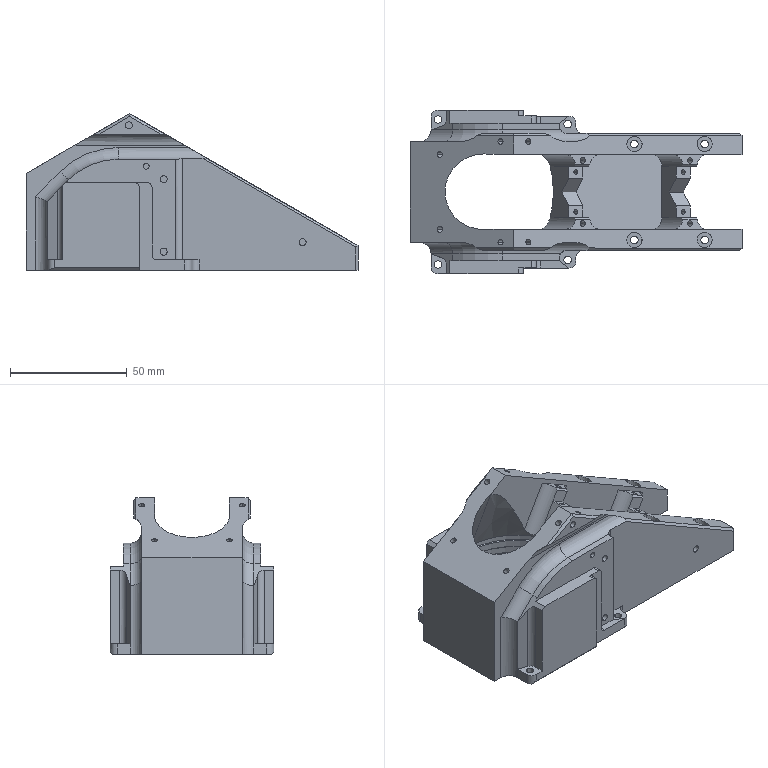NC program | NX | posted with a generic post | part box 142 x 70 x 67 mm
Lines 1 to 899 of 58889:
N10 G17 G21 G94 G90
(FACE_MILLING , TOOL : D80)
N12 T01 M6
N14 G54
N16 G17 G0 G90 X123. Y0. S2500 M3
N18 G43 Z33. H1
N20 G94 G1 Z0.3 F5000.
N22 X111. F1000.
N24 X-111.
N26 X-123.
N28 G0 Z33.
N30 M5
(DRILLING_COPY_2_COPY , TOOL : U钻-D21)
N32 T14 M6
N34 G54
N36 G17 G0 G90 X-36. Y0. S2000 M3
N38 G43 Z30. H14
N40 G94 G83 G99 Z-41. F100. Q2. R1.5
N42 G0 Z20.
N44 G80
N46 G0 X-36. Y0. Z30.
N48 M5
(PLANAR_MILL_COPY , TOOL : D16R0波刀)
N50 T02 M6
N52 G54
N54 G17 G0 G90 X87.25 Y8. S5500 M3
N56 G43 Z30.35 H2
N58 G94 G1 Z-2.65 F5000.
N60 G3 X79.25 Y0. R8. F2500.
N62 G1 Y-24.
N64 G2 X76.834 Y-29.834 R8.25
N66 G1 X75.834 Y-30.834
N68 G2 X70. Y-33.25 R8.25
N70 G1 X7.607
N72 G2 X-2.306 Y-40.729 R11.25
N74 G1 X-21.973 Y-43.25
N76 X-59.
N78 G2 X-70.25 Y-32. R11.25
N80 G1 Y-29.75
N82 X-71.
N84 G2 X-79.25 Y-21.5 R8.25
N86 G1 Y21.5
N88 G2 X-71. Y29.75 R8.25
N90 G1 X-70.25
N92 Y32.
N94 G2 X-59. Y43.25 R11.25
N96 G1 X-21.973
N98 X-2.306 Y40.729
N100 G2 X7.607 Y33.25 R11.25
N102 G1 X70.
N104 G2 X75.834 Y30.834 R8.25
N106 G1 X76.834 Y29.834
N108 G2 X79.25 Y24. R8.25
N110 G1 Y0.
N112 G3 X87.25 Y-8. R8.
N114 G0 Y8. Z-5.65
N116 G3 X79.25 Y0. R8.
N118 G1 Y-24.
N120 G2 X76.834 Y-29.834 R8.25
N122 G1 X75.834 Y-30.834
N124 G2 X70. Y-33.25 R8.25
N126 G1 X7.607
N128 G2 X-2.306 Y-40.729 R11.25
N130 G1 X-21.973 Y-43.25
N132 X-59.
N134 G2 X-70.25 Y-32. R11.25
N136 G1 Y-29.75
N138 X-71.
N140 G2 X-79.25 Y-21.5 R8.25
N142 G1 Y21.5
N144 G2 X-71. Y29.75 R8.25
N146 G1 X-70.25
N148 Y32.
N150 G2 X-59. Y43.25 R11.25
N152 G1 X-21.973
N154 X-2.306 Y40.729
N156 G2 X7.607 Y33.25 R11.25
N158 G1 X70.
N160 G2 X75.834 Y30.834 R8.25
N162 G1 X76.834 Y29.834
N164 G2 X79.25 Y24. R8.25
N166 G1 Y0.
N168 G3 X87.25 Y-8. R8.
N170 G0 Y8. Z-8.65
N172 G3 X79.25 Y0. R8.
N174 G1 Y-24.
N176 G2 X76.834 Y-29.834 R8.25
N178 G1 X75.834 Y-30.834
N180 G2 X70. Y-33.25 R8.25
N182 G1 X7.607
N184 G2 X-2.306 Y-40.729 R11.25
N186 G1 X-21.973 Y-43.25
N188 X-59.
N190 G2 X-70.25 Y-32. R11.25
N192 G1 Y-29.75
N194 X-71.
N196 G2 X-79.25 Y-21.5 R8.25
N198 G1 Y21.5
N200 G2 X-71. Y29.75 R8.25
N202 G1 X-70.25
N204 Y32.
N206 G2 X-59. Y43.25 R11.25
N208 G1 X-21.973
N210 X-2.306 Y40.729
N212 G2 X7.607 Y33.25 R11.25
N214 G1 X70.
N216 G2 X75.834 Y30.834 R8.25
N218 G1 X76.834 Y29.834
N220 G2 X79.25 Y24. R8.25
N222 G1 Y0.
N224 G3 X87.25 Y-8. R8.
N226 G0 Y8. Z-11.65
N228 G3 X79.25 Y0. R8.
N230 G1 Y-24.
N232 G2 X76.834 Y-29.834 R8.25
N234 G1 X75.834 Y-30.834
N236 G2 X70. Y-33.25 R8.25
N238 G1 X7.607
N240 G2 X-2.306 Y-40.729 R11.25
N242 G1 X-21.973 Y-43.25
N244 X-59.
N246 G2 X-70.25 Y-32. R11.25
N248 G1 Y-29.75
N250 X-71.
N252 G2 X-79.25 Y-21.5 R8.25
N254 G1 Y21.5
N256 G2 X-71. Y29.75 R8.25
N258 G1 X-70.25
N260 Y32.
N262 G2 X-59. Y43.25 R11.25
N264 G1 X-21.973
N266 X-2.306 Y40.729
N268 G2 X7.607 Y33.25 R11.25
N270 G1 X70.
N272 G2 X75.834 Y30.834 R8.25
N274 G1 X76.834 Y29.834
N276 G2 X79.25 Y24. R8.25
N278 G1 Y0.
N280 G3 X87.25 Y-8. R8.
N282 G0 Y8. Z-14.65
N284 G3 X79.25 Y0. R8.
N286 G1 Y-24.
N288 G2 X76.834 Y-29.834 R8.25
N290 G1 X75.834 Y-30.834
N292 G2 X70. Y-33.25 R8.25
N294 G1 X7.607
N296 G2 X-2.306 Y-40.729 R11.25
N298 G1 X-21.973 Y-43.25
N300 X-59.
N302 G2 X-70.25 Y-32. R11.25
N304 G1 Y-29.75
N306 X-71.
N308 G2 X-79.25 Y-21.5 R8.25
N310 G1 Y21.5
N312 G2 X-71. Y29.75 R8.25
N314 G1 X-70.25
N316 Y32.
N318 G2 X-59. Y43.25 R11.25
N320 G1 X-21.973
N322 X-2.306 Y40.729
N324 G2 X7.607 Y33.25 R11.25
N326 G1 X70.
N328 G2 X75.834 Y30.834 R8.25
N330 G1 X76.834 Y29.834
N332 G2 X79.25 Y24. R8.25
N334 G1 Y0.
N336 G3 X87.25 Y-8. R8.
N338 G0 Y8. Z-17.65
N340 G3 X79.25 Y0. R8.
N342 G1 Y-24.
N344 G2 X76.834 Y-29.834 R8.25
N346 G1 X75.834 Y-30.834
N348 G2 X70. Y-33.25 R8.25
N350 G1 X7.607
N352 G2 X-2.306 Y-40.729 R11.25
N354 G1 X-21.973 Y-43.25
N356 X-59.
N358 G2 X-70.25 Y-32. R11.25
N360 G1 Y-29.75
N362 X-71.
N364 G2 X-79.25 Y-21.5 R8.25
N366 G1 Y21.5
N368 G2 X-71. Y29.75 R8.25
N370 G1 X-70.25
N372 Y32.
N374 G2 X-59. Y43.25 R11.25
N376 G1 X-21.973
N378 X-2.306 Y40.729
N380 G2 X7.607 Y33.25 R11.25
N382 G1 X70.
N384 G2 X75.834 Y30.834 R8.25
N386 G1 X76.834 Y29.834
N388 G2 X79.25 Y24. R8.25
N390 G1 Y0.
N392 G3 X87.25 Y-8. R8.
N394 G0 Y8. Z-20.65
N396 G3 X79.25 Y0. R8.
N398 G1 Y-24.
N400 G2 X76.834 Y-29.834 R8.25
N402 G1 X75.834 Y-30.834
N404 G2 X70. Y-33.25 R8.25
N406 G1 X7.607
N408 G2 X-2.306 Y-40.729 R11.25
N410 G1 X-21.973 Y-43.25
N412 X-59.
N414 G2 X-70.25 Y-32. R11.25
N416 G1 Y-29.75
N418 X-71.
N420 G2 X-79.25 Y-21.5 R8.25
N422 G1 Y21.5
N424 G2 X-71. Y29.75 R8.25
N426 G1 X-70.25
N428 Y32.
N430 G2 X-59. Y43.25 R11.25
N432 G1 X-21.973
N434 X-2.306 Y40.729
N436 G2 X7.607 Y33.25 R11.25
N438 G1 X70.
N440 G2 X75.834 Y30.834 R8.25
N442 G1 X76.834 Y29.834
N444 G2 X79.25 Y24. R8.25
N446 G1 Y0.
N448 G3 X87.25 Y-8. R8.
N450 G0 Y8. Z-23.65
N452 G3 X79.25 Y0. R8.
N454 G1 Y-24.
N456 G2 X76.834 Y-29.834 R8.25
N458 G1 X75.834 Y-30.834
N460 G2 X70. Y-33.25 R8.25
N462 G1 X7.607
N464 G2 X-2.306 Y-40.729 R11.25
N466 G1 X-21.973 Y-43.25
N468 X-59.
N470 G2 X-70.25 Y-32. R11.25
N472 G1 Y-29.75
N474 X-71.
N476 G2 X-79.25 Y-21.5 R8.25
N478 G1 Y21.5
N480 G2 X-71. Y29.75 R8.25
N482 G1 X-70.25
N484 Y32.
N486 G2 X-59. Y43.25 R11.25
N488 G1 X-21.973
N490 X-2.306 Y40.729
N492 G2 X7.607 Y33.25 R11.25
N494 G1 X70.
N496 G2 X75.834 Y30.834 R8.25
N498 G1 X76.834 Y29.834
N500 G2 X79.25 Y24. R8.25
N502 G1 Y0.
N504 G3 X87.25 Y-8. R8.
N506 G0 Y8. Z-26.65
N508 G3 X79.25 Y0. R8.
N510 G1 Y-24.
N512 G2 X76.834 Y-29.834 R8.25
N514 G1 X75.834 Y-30.834
N516 G2 X70. Y-33.25 R8.25
N518 G1 X7.607
N520 G2 X-2.306 Y-40.729 R11.25
N522 G1 X-21.973 Y-43.25
N524 X-59.
N526 G2 X-70.25 Y-32. R11.25
N528 G1 Y-29.75
N530 X-71.
N532 G2 X-79.25 Y-21.5 R8.25
N534 G1 Y21.5
N536 G2 X-71. Y29.75 R8.25
N538 G1 X-70.25
N540 Y32.
N542 G2 X-59. Y43.25 R11.25
N544 G1 X-21.973
N546 X-2.306 Y40.729
N548 G2 X7.607 Y33.25 R11.25
N550 G1 X70.
N552 G2 X75.834 Y30.834 R8.25
N554 G1 X76.834 Y29.834
N556 G2 X79.25 Y24. R8.25
N558 G1 Y0.
N560 G3 X87.25 Y-8. R8.
N562 G0 Y8. Z-29.65
N564 G3 X79.25 Y0. R8.
N566 G1 Y-24.
N568 G2 X76.834 Y-29.834 R8.25
N570 G1 X75.834 Y-30.834
N572 G2 X70. Y-33.25 R8.25
N574 G1 X7.607
N576 G2 X-2.306 Y-40.729 R11.25
N578 G1 X-21.973 Y-43.25
N580 X-59.
N582 G2 X-70.25 Y-32. R11.25
N584 G1 Y-29.75
N586 X-71.
N588 G2 X-79.25 Y-21.5 R8.25
N590 G1 Y21.5
N592 G2 X-71. Y29.75 R8.25
N594 G1 X-70.25
N596 Y32.
N598 G2 X-59. Y43.25 R11.25
N600 G1 X-21.973
N602 X-2.306 Y40.729
N604 G2 X7.607 Y33.25 R11.25
N606 G1 X70.
N608 G2 X75.834 Y30.834 R8.25
N610 G1 X76.834 Y29.834
N612 G2 X79.25 Y24. R8.25
N614 G1 Y0.
N616 G3 X87.25 Y-8. R8.
N618 G0 Y8. Z-32.65
N620 G3 X79.25 Y0. R8.
N622 G1 Y-24.
N624 G2 X76.834 Y-29.834 R8.25
N626 G1 X75.834 Y-30.834
N628 G2 X70. Y-33.25 R8.25
N630 G1 X7.607
N632 G2 X-2.306 Y-40.729 R11.25
N634 G1 X-21.973 Y-43.25
N636 X-59.
N638 G2 X-70.25 Y-32. R11.25
N640 G1 Y-29.75
N642 X-71.
N644 G2 X-79.25 Y-21.5 R8.25
N646 G1 Y21.5
N648 G2 X-71. Y29.75 R8.25
N650 G1 X-70.25
N652 Y32.
N654 G2 X-59. Y43.25 R11.25
N656 G1 X-21.973
N658 X-2.306 Y40.729
N660 G2 X7.607 Y33.25 R11.25
N662 G1 X70.
N664 G2 X75.834 Y30.834 R8.25
N666 G1 X76.834 Y29.834
N668 G2 X79.25 Y24. R8.25
N670 G1 Y0.
N672 G3 X87.25 Y-8. R8.
N674 G0 Y8. Z-35.65
N676 G3 X79.25 Y0. R8.
N678 G1 Y-24.
N680 G2 X76.834 Y-29.834 R8.25
N682 G1 X75.834 Y-30.834
N684 G2 X70. Y-33.25 R8.25
N686 G1 X7.607
N688 G2 X-2.306 Y-40.729 R11.25
N690 G1 X-21.973 Y-43.25
N692 X-59.
N694 G2 X-70.25 Y-32. R11.25
N696 G1 Y-29.75
N698 X-71.
N700 G2 X-79.25 Y-21.5 R8.25
N702 G1 Y21.5
N704 G2 X-71. Y29.75 R8.25
N706 G1 X-70.25
N708 Y32.
N710 G2 X-59. Y43.25 R11.25
N712 G1 X-21.973
N714 X-2.306 Y40.729
N716 G2 X7.607 Y33.25 R11.25
N718 G1 X70.
N720 G2 X75.834 Y30.834 R8.25
N722 G1 X76.834 Y29.834
N724 G2 X79.25 Y24. R8.25
N726 G1 Y0.
N728 G3 X87.25 Y-8. R8.
N730 G0 Y8. Z-38.65
N732 G3 X79.25 Y0. R8.
N734 G1 Y-24.
N736 G2 X76.834 Y-29.834 R8.25
N738 G1 X75.834 Y-30.834
N740 G2 X70. Y-33.25 R8.25
N742 G1 X7.607
N744 G2 X-2.306 Y-40.729 R11.25
N746 G1 X-21.973 Y-43.25
N748 X-59.
N750 G2 X-70.25 Y-32. R11.25
N752 G1 Y-29.75
N754 X-71.
N756 G2 X-79.25 Y-21.5 R8.25
N758 G1 Y21.5
N760 G2 X-71. Y29.75 R8.25
N762 G1 X-70.25
N764 Y32.
N766 G2 X-59. Y43.25 R11.25
N768 G1 X-21.973
N770 X-2.306 Y40.729
N772 G2 X7.607 Y33.25 R11.25
N774 G1 X70.
N776 G2 X75.834 Y30.834 R8.25
N778 G1 X76.834 Y29.834
N780 G2 X79.25 Y24. R8.25
N782 G1 Y0.
N784 G3 X87.25 Y-8. R8.
N786 G0 Y8. Z-41.65
N788 G3 X79.25 Y0. R8.
N790 G1 Y-24.
N792 G2 X76.834 Y-29.834 R8.25
N794 G1 X75.834 Y-30.834
N796 G2 X70. Y-33.25 R8.25
N798 G1 X7.607
N800 G2 X-2.306 Y-40.729 R11.25
N802 G1 X-21.973 Y-43.25
N804 X-59.
N806 G2 X-70.25 Y-32. R11.25
N808 G1 Y-29.75
N810 X-71.
N812 G2 X-79.25 Y-21.5 R8.25
N814 G1 Y21.5
N816 G2 X-71. Y29.75 R8.25
N818 G1 X-70.25
N820 Y32.
N822 G2 X-59. Y43.25 R11.25
N824 G1 X-21.973
N826 X-2.306 Y40.729
N828 G2 X7.607 Y33.25 R11.25
N830 G1 X70.
N832 G2 X75.834 Y30.834 R8.25
N834 G1 X76.834 Y29.834
N836 G2 X79.25 Y24. R8.25
N838 G1 Y0.
N840 G3 X87.25 Y-8. R8.
N842 G0 Y8. Z-44.65
N844 G3 X79.25 Y0. R8.
N846 G1 Y-24.
N848 G2 X76.834 Y-29.834 R8.25
N850 G1 X75.834 Y-30.834
N852 G2 X70. Y-33.25 R8.25
N854 G1 X7.607
N856 G2 X-2.306 Y-40.729 R11.25
N858 G1 X-21.973 Y-43.25
N860 X-59.
N862 G2 X-70.25 Y-32. R11.25
N864 G1 Y-29.75
N866 X-71.
N868 G2 X-79.25 Y-21.5 R8.25
N870 G1 Y21.5
N872 G2 X-71. Y29.75 R8.25
N874 G1 X-70.25
N876 Y32.
N878 G2 X-59. Y43.25 R11.25
N880 G1 X-21.973
N882 X-2.306 Y40.729
N884 G2 X7.607 Y33.25 R11.25
N886 G1 X70.
N888 G2 X75.834 Y30.834 R8.25
N890 G1 X76.834 Y29.834
N892 G2 X79.25 Y24. R8.25
N894 G1 Y0.
N896 G3 X87.25 Y-8. R8.
N898 G0 Y8. Z-47.65
N900 G3 X79.25 Y0. R8.
N902 G1 Y-24.
N904 G2 X76.834 Y-29.834 R8.25
N906 G1 X75.834 Y-30.834
N908 G2 X70. Y-33.25 R8.25
N910 G1 X7.607
N912 G2 X-2.306 Y-40.729 R11.25
N914 G1 X-21.973 Y-43.25
N916 X-59.
N918 G2 X-70.25 Y-32. R11.25
N920 G1 Y-29.75
N922 X-71.
N924 G2 X-79.25 Y-21.5 R8.25
N926 G1 Y21.5
N928 G2 X-71. Y29.75 R8.25
N930 G1 X-70.25
N932 Y32.
N934 G2 X-59. Y43.25 R11.25
N936 G1 X-21.973
N938 X-2.306 Y40.729
N940 G2 X7.607 Y33.25 R11.25
N942 G1 X70.
N944 G2 X75.834 Y30.834 R8.25
N946 G1 X76.834 Y29.834
N948 G2 X79.25 Y24. R8.25
N950 G1 Y0.
N952 G3 X87.25 Y-8. R8.
N954 G0 Y8. Z-50.65
N956 G3 X79.25 Y0. R8.
N958 G1 Y-24.
N960 G2 X76.834 Y-29.834 R8.25
N962 G1 X75.834 Y-30.834
N964 G2 X70. Y-33.25 R8.25
N966 G1 X7.607
N968 G2 X-2.306 Y-40.729 R11.25
N970 G1 X-21.973 Y-43.25
N972 X-59.
N974 G2 X-70.25 Y-32. R11.25
N976 G1 Y-29.75
N978 X-71.
N980 G2 X-79.25 Y-21.5 R8.25
N982 G1 Y21.5
N984 G2 X-71. Y29.75 R8.25
N986 G1 X-70.25
N988 Y32.
N990 G2 X-59. Y43.25 R11.25
N992 G1 X-21.973
N994 X-2.306 Y40.729
N996 G2 X7.607 Y33.25 R11.25
N998 G1 X70.
N1000 G2 X75.834 Y30.834 R8.25
N1002 G1 X76.834 Y29.834
N1004 G2 X79.25 Y24. R8.25
N1006 G1 Y0.
N1008 G3 X87.25 Y-8. R8.
N1010 G0 Y8. Z-53.65
N1012 G3 X79.25 Y0. R8.
N1014 G1 Y-24.
N1016 G2 X76.834 Y-29.834 R8.25
N1018 G1 X75.834 Y-30.834
N1020 G2 X70. Y-33.25 R8.25
N1022 G1 X7.607
N1024 G2 X-2.306 Y-40.729 R11.25
N1026 G1 X-21.973 Y-43.25
N1028 X-59.
N1030 G2 X-70.25 Y-32. R11.25
N1032 G1 Y-29.75
N1034 X-71.
N1036 G2 X-79.25 Y-21.5 R8.25
N1038 G1 Y21.5
N1040 G2 X-71. Y29.75 R8.25
N1042 G1 X-70.25
N1044 Y32.
N1046 G2 X-59. Y43.25 R11.25
N1048 G1 X-21.973
N1050 X-2.306 Y40.729
N1052 G2 X7.607 Y33.25 R11.25
N1054 G1 X70.
N1056 G2 X75.834 Y30.834 R8.25
N1058 G1 X76.834 Y29.834
N1060 G2 X79.25 Y24. R8.25
N1062 G1 Y0.
N1064 G3 X87.25 Y-8. R8.
N1066 G0 Y8. Z-56.65
N1068 G3 X79.25 Y0. R8.
N1070 G1 Y-24.
N1072 G2 X76.834 Y-29.834 R8.25
N1074 G1 X75.834 Y-30.834
N1076 G2 X70. Y-33.25 R8.25
N1078 G1 X7.607
N1080 G2 X-2.306 Y-40.729 R11.25
N1082 G1 X-21.973 Y-43.25
N1084 X-59.
N1086 G2 X-70.25 Y-32. R11.25
N1088 G1 Y-29.75
N1090 X-71.
N1092 G2 X-79.25 Y-21.5 R8.25
N1094 G1 Y21.5
N1096 G2 X-71. Y29.75 R8.25
N1098 G1 X-70.25
N1100 Y32.
N1102 G2 X-59. Y43.25 R11.25
N1104 G1 X-21.973
N1106 X-2.306 Y40.729
N1108 G2 X7.607 Y33.25 R11.25
N1110 G1 X70.
N1112 G2 X75.834 Y30.834 R8.25
N1114 G1 X76.834 Y29.834
N1116 G2 X79.25 Y24. R8.25
N1118 G1 Y0.
N1120 G3 X87.25 Y-8. R8.
N1122 G0 Y8. Z-59.65
N1124 G3 X79.25 Y0. R8.
N1126 G1 Y-24.
N1128 G2 X76.834 Y-29.834 R8.25
N1130 G1 X75.834 Y-30.834
N1132 G2 X70. Y-33.25 R8.25
N1134 G1 X7.607
N1136 G2 X-2.306 Y-40.729 R11.25
N1138 G1 X-21.973 Y-43.25
N1140 X-59.
N1142 G2 X-70.25 Y-32. R11.25
N1144 G1 Y-29.75
N1146 X-71.
N1148 G2 X-79.25 Y-21.5 R8.25
N1150 G1 Y21.5
N1152 G2 X-71. Y29.75 R8.25
N1154 G1 X-70.25
N1156 Y32.
N1158 G2 X-59. Y43.25 R11.25
N1160 G1 X-21.973
N1162 X-2.306 Y40.729
N1164 G2 X7.607 Y33.25 R11.25
N1166 G1 X70.
N1168 G2 X75.834 Y30.834 R8.25
N1170 G1 X76.834 Y29.834
N1172 G2 X79.25 Y24. R8.25
N1174 G1 Y0.
N1176 G3 X87.25 Y-8. R8.
N1178 G0 Y8. Z-62.65
N1180 G3 X79.25 Y0. R8.
N1182 G1 Y-24.
N1184 G2 X76.834 Y-29.834 R8.25
N1186 G1 X75.834 Y-30.834
N1188 G2 X70. Y-33.25 R8.25
N1190 G1 X7.607
N1192 G2 X-2.306 Y-40.729 R11.25
N1194 G1 X-21.973 Y-43.25
N1196 X-59.
N1198 G2 X-70.25 Y-32. R11.25
N1200 G1 Y-29.75
N1202 X-71.
N1204 G2 X-79.25 Y-21.5 R8.25
N1206 G1 Y21.5
N1208 G2 X-71. Y29.75 R8.25
N1210 G1 X-70.25
N1212 Y32.
N1214 G2 X-59. Y43.25 R11.25
N1216 G1 X-21.973
N1218 X-2.306 Y40.729
N1220 G2 X7.607 Y33.25 R11.25
N1222 G1 X70.
N1224 G2 X75.834 Y30.834 R8.25
N1226 G1 X76.834 Y29.834
N1228 G2 X79.25 Y24. R8.25
N1230 G1 Y0.
N1232 G3 X87.25 Y-8. R8.
N1234 G0 Y8. Z-65.65
N1236 G3 X79.25 Y0. R8.
N1238 G1 Y-24.
N1240 G2 X76.834 Y-29.834 R8.25
N1242 G1 X75.834 Y-30.834
N1244 G2 X70. Y-33.25 R8.25
N1246 G1 X7.607
N1248 G2 X-2.306 Y-40.729 R11.25
N1250 G1 X-21.973 Y-43.25
N1252 X-59.
N1254 G2 X-70.25 Y-32. R11.25
N1256 G1 Y-29.75
N1258 X-71.
N1260 G2 X-79.25 Y-21.5 R8.25
N1262 G1 Y21.5
N1264 G2 X-71. Y29.75 R8.25
N1266 G1 X-70.25
N1268 Y32.
N1270 G2 X-59. Y43.25 R11.25
N1272 G1 X-21.973
N1274 X-2.306 Y40.729
N1276 G2 X7.607 Y33.25 R11.25
N1278 G1 X70.
N1280 G2 X75.834 Y30.834 R8.25
N1282 G1 X76.834 Y29.834
N1284 G2 X79.25 Y24. R8.25
N1286 G1 Y0.
N1288 G3 X87.25 Y-8. R8.
N1290 G0 Y8. Z-67.3
N1292 G3 X79.25 Y0. R8.
N1294 G1 Y-24.
N1296 G2 X76.834 Y-29.834 R8.25
N1298 G1 X75.834 Y-30.834
N1300 G2 X70. Y-33.25 R8.25
N1302 G1 X7.607
N1304 G2 X-2.306 Y-40.729 R11.25
N1306 G1 X-21.973 Y-43.25
N1308 X-59.
N1310 G2 X-70.25 Y-32. R11.25
N1312 G1 Y-29.75
N1314 X-71.
N1316 G2 X-79.25 Y-21.5 R8.25
N1318 G1 Y21.5
N1320 G2 X-71. Y29.75 R8.25
N1322 G1 X-70.25
N1324 Y32.
N1326 G2 X-59. Y43.25 R11.25
N1328 G1 X-21.973
N1330 X-2.306 Y40.729
N1332 G2 X7.607 Y33.25 R11.25
N1334 G1 X70.
N1336 G2 X75.834 Y30.834 R8.25
N1338 G1 X76.834 Y29.834
N1340 G2 X79.25 Y24. R8.25
N1342 G1 Y0.
N1344 G3 X87.25 Y-8. R8.
N1346 G0 Z30.35
(PLANAR_MILL_COPY_COPY_2 , TOOL : D16R0波刀)
N1348 X-36. Y0.1
N1350 Z30.3
N1352 G1 Z-2.2 F5000.
N1354 Y6.5 F2000.
N1356 X-41.347
N1358 G3 X-41.347 Y-6.5 R7.402
N1360 G1 X-20.31
N1362 G3 X-20.304 Y6.5 R23.684
N1364 G1 X-36.
N1366 Y0.1
N1368 G0 Z-4.7
N1370 G1 Y6.5
N1372 X-41.347
N1374 G3 X-41.347 Y-6.5 R7.402
N1376 G1 X-20.31
N1378 G3 X-20.304 Y6.5 R23.684
N1380 G1 X-36.
N1382 Y0.1
N1384 G0 Z-7.2
N1386 G1 Y6.5
N1388 X-41.347
N1390 G3 X-41.347 Y-6.5 R7.402
N1392 G1 X-20.31
N1394 G3 X-20.304 Y6.5 R23.684
N1396 G1 X-36.
N1398 Y0.1
N1400 G0 Z-9.7
N1402 G1 Y6.5
N1404 X-41.347
N1406 G3 X-41.347 Y-6.5 R7.402
N1408 G1 X-20.31
N1410 G3 X-20.304 Y6.5 R23.684
N1412 G1 X-36.
N1414 Y0.1
N1416 G0 Z-12.2
N1418 G1 Y6.5
N1420 X-41.347
N1422 G3 X-41.347 Y-6.5 R7.402
N1424 G1 X-20.31
N1426 G3 X-20.304 Y6.5 R23.684
N1428 G1 X-36.
N1430 Y0.1
N1432 G0 Z-14.7
N1434 G1 Y6.5
N1436 X-41.347
N1438 G3 X-41.347 Y-6.5 R7.402
N1440 G1 X-20.31
N1442 G3 X-20.304 Y6.5 R23.684
N1444 G1 X-36.
N1446 Y0.1
N1448 G0 Z-17.2
N1450 G1 Y6.5
N1452 X-41.347
N1454 G3 X-41.347 Y-6.5 R7.402
N1456 G1 X-20.31
N1458 G3 X-20.304 Y6.5 R23.684
N1460 G1 X-36.
N1462 Y0.1
N1464 G0 Z-19.7
N1466 G1 Y6.5
N1468 X-41.347
N1470 G3 X-41.347 Y-6.5 R7.402
N1472 G1 X-20.31
N1474 G3 X-20.304 Y6.5 R23.684
N1476 G1 X-36.
N1478 Y0.1
N1480 G0 Z-22.2
N1482 G1 Y6.5
N1484 X-41.347
N1486 G3 X-41.347 Y-6.5 R7.402
N1488 G1 X-20.31
N1490 G3 X-20.304 Y6.5 R23.684
N1492 G1 X-36.
N1494 Y0.1
N1496 G0 Z-24.7
N1498 G1 Y6.5
N1500 X-41.347
N1502 G3 X-41.347 Y-6.5 R7.402
N1504 G1 X-20.31
N1506 G3 X-20.304 Y6.5 R23.684
N1508 G1 X-36.
N1510 Y0.1
N1512 G0 Z-27.2
N1514 G1 Y6.5
N1516 X-41.347
N1518 G3 X-41.347 Y-6.5 R7.402
N1520 G1 X-20.31
N1522 G3 X-20.304 Y6.5 R23.684
N1524 G1 X-36.
N1526 Y0.1
N1528 G0 Z-29.7
N1530 G1 Y6.5
N1532 X-41.347
N1534 G3 X-41.347 Y-6.5 R7.402
N1536 G1 X-20.31
N1538 G3 X-20.304 Y6.5 R23.684
N1540 G1 X-36.
N1542 Y0.1
N1544 G0 Z-32.2
N1546 G1 Y6.5
N1548 X-41.347
N1550 G3 X-41.347 Y-6.5 R7.402
N1552 G1 X-20.31
N1554 G3 X-20.304 Y6.5 R23.684
N1556 G1 X-36.
N1558 Y0.1
N1560 G0 Z-34.7
N1562 G1 Y6.5
N1564 X-41.347
N1566 G3 X-41.347 Y-6.5 R7.402
N1568 G1 X-20.31
N1570 G3 X-20.304 Y6.5 R23.684
N1572 G1 X-36.
N1574 Y0.1
N1576 G0 Z-37.2
N1578 G1 Y6.5
N1580 X-41.347
N1582 G3 X-41.347 Y-6.5 R7.402
N1584 G1 X-20.31
N1586 G3 X-20.304 Y6.5 R23.684
N1588 G1 X-36.
N1590 Y0.1
N1592 G0 Z-39.
N1594 G1 Y6.5
N1596 X-41.347
N1598 G3 X-41.347 Y-6.5 R7.402
N1600 G1 X-20.31
N1602 G3 X-20.304 Y6.5 R23.684
N1604 G1 X-36.
N1606 Y0.1
N1608 G0 Z30.3
(PLANAR_MILL_COPY_COPY_3 , TOOL : D16R0波刀)
N1610 X82.2 Y6.
N1612 Z30.
N1614 G1 Z-3. F5000.
N1616 X71. F2500.
N1618 X61.
N1620 Y-6.
N1622 X71.
N1624 X82.2
N1626 G0 Y6. Z-6.
N1628 G1 X71.
N1630 X61.
N1632 Y-6.
N1634 X71.
N1636 X82.2
N1638 G0 Y6. Z-9.
N1640 G1 X71.
N1642 X61.
N1644 Y-6.
N1646 X71.
N1648 X82.2
N1650 G0 Y6. Z-12.
N1652 G1 X71.
N1654 X61.
N1656 Y-6.
N1658 X71.
N1660 X82.2
N1662 G0 Y6. Z-15.
N1664 G1 X71.
N1666 X61.
N1668 Y-6.
N1670 X71.
N1672 X82.2
N1674 G0 Y6. Z-18.
N1676 G1 X71.
N1678 X61.
N1680 Y-6.
N1682 X71.
N1684 X82.2
N1686 G0 Y6. Z-21.
N1688 G1 X71.
N1690 X61.
N1692 Y-6.
N1694 X71.
N1696 X82.2
N1698 G0 Y6. Z-24.
N1700 G1 X71.
N1702 X61.
N1704 Y-6.
N1706 X71.
N1708 X82.2
N1710 G0 Y6. Z-27.
N1712 G1 X71.
N1714 X61.
N1716 Y-6.
N1718 X71.
N1720 X82.2
N1722 G0 Y6. Z-30.
N1724 G1 X71.
N1726 X61.
N1728 Y-6.
N1730 X71.
N1732 X82.2
N1734 G0 Y6. Z-33.
N1736 G1 X71.
N1738 X61.
N1740 Y-6.
N1742 X71.
N1744 X82.2
N1746 G0 Y6. Z-36.
N1748 G1 X71.
N1750 X61.
N1752 Y-6.
N1754 X71.
N1756 X82.2
N1758 G0 Y6. Z-38.
N1760 G1 X71.
N1762 X61.
N1764 Y-6.
N1766 X71.
N1768 X82.2
N1770 G0 Z30.
N1772 M5